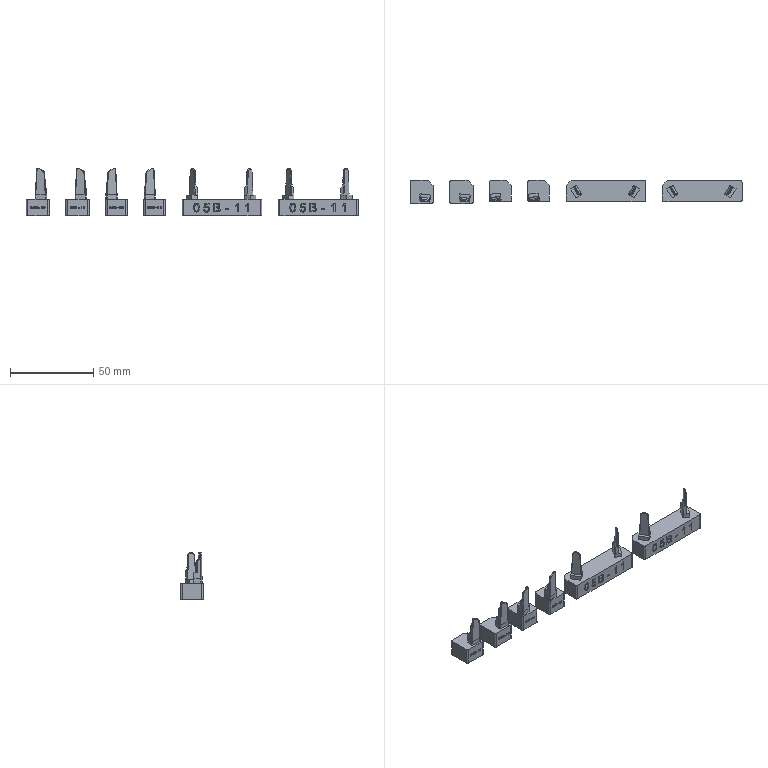Part | 6 solids | 618 faces | box 200 x 14 x 28.763 mm | volume 21220 mm3 | plane 284 | spline 284 | cylinder 50 | commonest cylinder face diameters 2 x18 0.603 x16 4.02 x12 2.01 x4